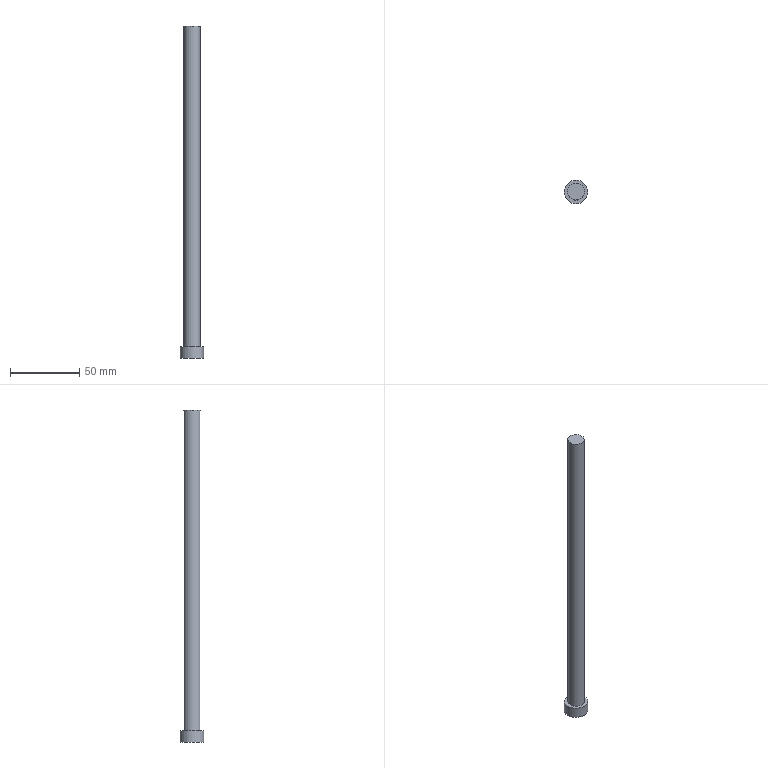Part | NX | features 模具.stp<1>[100] 2 | 1 solid | 5 faces | box 17 x 17 x 239.5 mm | volume 27998 mm3 | plane 3 | cylinder 2 | commonest cylinder face diameters 12 x1 17 x1
STEP:
#1=CARTESIAN_POINT('',(109.,-54.,24.));
#2=VERTEX_POINT('',#1);
#3=CARTESIAN_POINT('',(115.,-54.,24.));
#4=DIRECTION('',(0.,0.,-1.));
#5=DIRECTION('',(-1.,0.,0.));
#6=AXIS2_PLACEMENT_3D('',#3,#4,#5);
#7=CIRCLE('',#6,6.);
#8=EDGE_CURVE('',#2,#2,#7,.T.);
#9=ORIENTED_EDGE('',*,*,#8,.F.);
#10=EDGE_LOOP('',(#9));
#11=FACE_BOUND('',#10,.T.);
#12=CARTESIAN_POINT('',(0.,0.,24.));
#13=DIRECTION('',(0.,0.,-1.));
#14=DIRECTION('',(0.,-1.,0.));
#15=AXIS2_PLACEMENT_3D('',#12,#13,#14);
#16=PLANE('',#15);
#17=ADVANCED_FACE('',(#11),#16,.F.);
#18=CARTESIAN_POINT('',(123.5,-54.,-215.5));
#19=VERTEX_POINT('',#18);
#20=CARTESIAN_POINT('',(115.,-54.,-215.5));
#21=DIRECTION('',(0.,0.,1.));
#22=DIRECTION('',(1.,0.,0.));
#23=AXIS2_PLACEMENT_3D('',#20,#21,#22);
#24=CIRCLE('',#23,8.5);
#25=EDGE_CURVE('',#19,#19,#24,.T.);
#26=ORIENTED_EDGE('',*,*,#25,.T.);
#27=EDGE_LOOP('',(#26));
#28=FACE_BOUND('',#27,.T.);
#29=CARTESIAN_POINT('',(123.5,-54.,-207.5));
#30=VERTEX_POINT('',#29);
#31=CARTESIAN_POINT('',(115.,-54.,-207.5));
#32=DIRECTION('',(0.,0.,-1.));
#33=DIRECTION('',(1.,0.,0.));
#34=AXIS2_PLACEMENT_3D('',#31,#32,#33);
#35=CIRCLE('',#34,8.5);
#36=EDGE_CURVE('',#30,#30,#35,.T.);
#37=ORIENTED_EDGE('',*,*,#36,.T.);
#38=EDGE_LOOP('',(#37));
#39=FACE_BOUND('',#38,.T.);
#40=CARTESIAN_POINT('',(115.,-54.,-215.5));
#41=DIRECTION('',(0.,0.,1.));
#42=DIRECTION('',(1.,0.,0.));
#43=AXIS2_PLACEMENT_3D('',#40,#41,#42);
#44=CYLINDRICAL_SURFACE('',#43,8.5);
#45=ADVANCED_FACE('',(#28,#39),#44,.T.);
#46=ORIENTED_EDGE('',*,*,#25,.F.);
#47=EDGE_LOOP('',(#46));
#48=FACE_BOUND('',#47,.T.);
#49=CARTESIAN_POINT('',(115.,-54.,-215.5));
#50=DIRECTION('',(0.,0.,-1.));
#51=DIRECTION('',(0.,-1.,0.));
#52=AXIS2_PLACEMENT_3D('',#49,#50,#51);
#53=PLANE('',#52);
#54=ADVANCED_FACE('',(#48),#53,.T.);
#55=ORIENTED_EDGE('',*,*,#36,.F.);
#56=EDGE_LOOP('',(#55));
#57=FACE_BOUND('',#56,.T.);
#58=CARTESIAN_POINT('',(121.,-54.,-207.5));
#59=VERTEX_POINT('',#58);
#60=CARTESIAN_POINT('',(115.,-54.,-207.5));
#61=DIRECTION('',(0.,0.,1.));
#62=DIRECTION('',(1.,0.,0.));
#63=AXIS2_PLACEMENT_3D('',#60,#61,#62);
#64=CIRCLE('',#63,6.);
#65=EDGE_CURVE('',#59,#59,#64,.T.);
#66=ORIENTED_EDGE('',*,*,#65,.F.);
#67=EDGE_LOOP('',(#66));
#68=FACE_BOUND('',#67,.T.);
#69=CARTESIAN_POINT('',(115.,-54.,-207.5));
#70=DIRECTION('',(0.,0.,1.));
#71=DIRECTION('',(1.,0.,0.));
#72=AXIS2_PLACEMENT_3D('',#69,#70,#71);
#73=PLANE('',#72);
#74=ADVANCED_FACE('',(#57,#68),#73,.T.);
#75=ORIENTED_EDGE('',*,*,#8,.T.);
#76=EDGE_LOOP('',(#75));
#77=FACE_BOUND('',#76,.T.);
#78=ORIENTED_EDGE('',*,*,#65,.T.);
#79=EDGE_LOOP('',(#78));
#80=FACE_BOUND('',#79,.T.);
#81=CARTESIAN_POINT('',(115.,-54.,-215.5));
#82=DIRECTION('',(0.,0.,1.));
#83=DIRECTION('',(1.,0.,0.));
#84=AXIS2_PLACEMENT_3D('',#81,#82,#83);
#85=CYLINDRICAL_SURFACE('',#84,6.);
#86=ADVANCED_FACE('',(#77,#80),#85,.T.);
#87=CLOSED_SHELL('',(#17,#45,#54,#74,#86));
#88=MANIFOLD_SOLID_BREP('',#87);
#89=(LENGTH_UNIT()NAMED_UNIT(*)SI_UNIT(.MILLI.,.METRE.));
#90=UNCERTAINTY_MEASURE_WITH_UNIT(LENGTH_MEASURE(0.00001),#89,'','');
#91=(NAMED_UNIT(*)PLANE_ANGLE_UNIT()SI_UNIT($,.RADIAN.));
#92=(NAMED_UNIT(*)SI_UNIT($,.STERADIAN.)SOLID_ANGLE_UNIT());
#93=(GEOMETRIC_REPRESENTATION_CONTEXT(3)GLOBAL_UNCERTAINTY_ASSIGNED_CONTEXT((#90))GLOBAL_UNIT_ASSIGNED_CONTEXT((#89,#91,#92))REPRESENTATION_CONTEXT('',''));
#94=ADVANCED_BREP_SHAPE_REPRESENTATION('',(#88),#93);